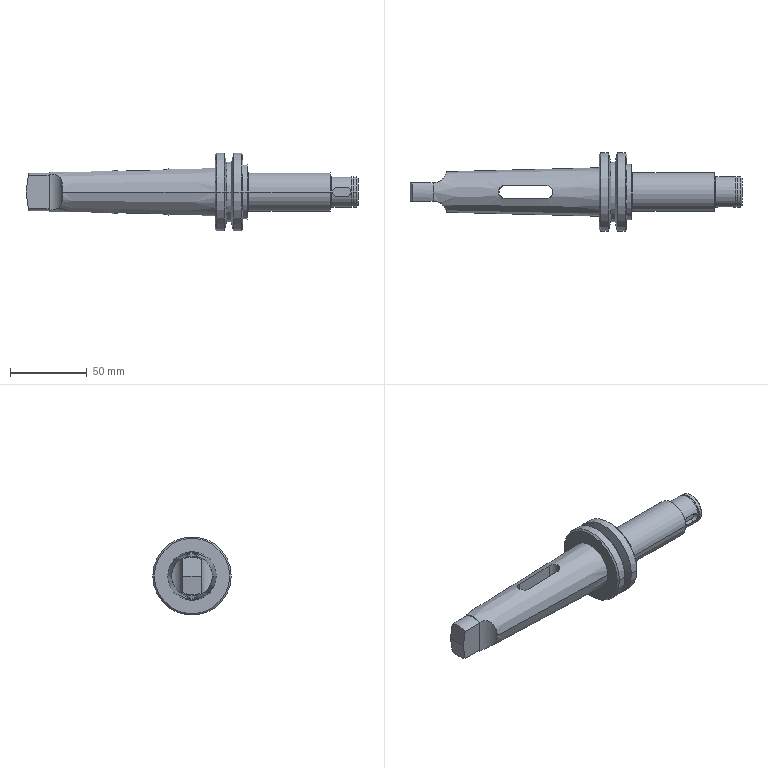Part | SolidWorks | features ICE 5, Chamfer 1, MirrorPattern 1, Revolution 1, SweepCut 1 | 1 solid | 62 faces | box 216 x 51 x 51 mm | volume 132474 mm3 | cylinder 28 | plane 20 | cone 12 | spline 2 | commonest cylinder face diameters 19 x4 20 x4 51 x4 6 x2 8.2 x2 18 x2